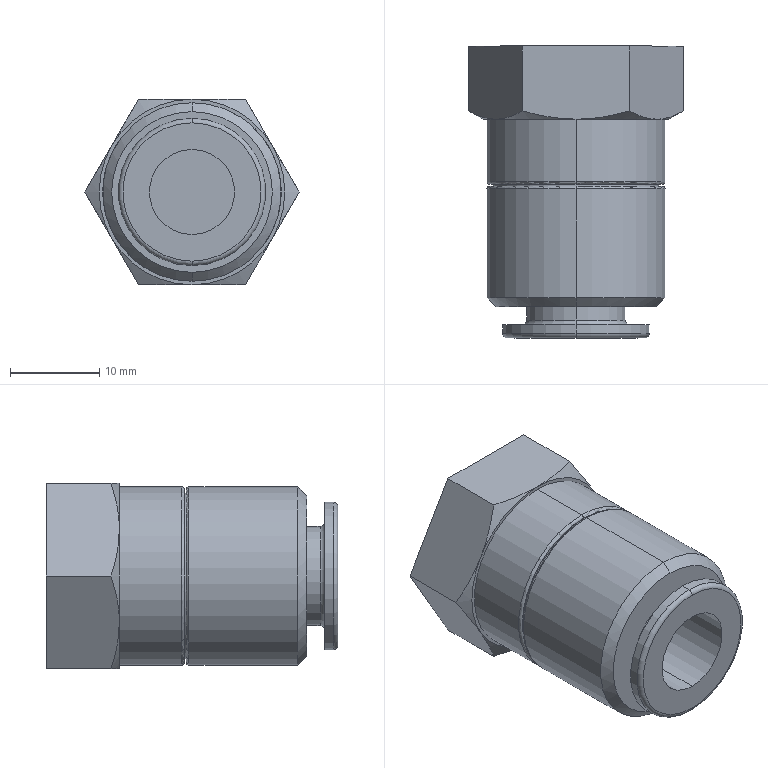Part | SolidWorks | features BaseBody 1 | 1 solid | 42 faces | box 23.995 x 32.7 x 20.78 mm | volume 9079 mm3 | plane 14 | cylinder 12 | torus 8 | cone 8 | commonest cylinder face diameters 20 x4 9.525 x2 11.1 x2 16.5 x2 18.56 x2
STEP:
#1=CARTESIAN_POINT('',(0.,-18.,4.763));
#2=VERTEX_POINT('',#1);
#3=CARTESIAN_POINT('',(0.,-18.,-4.763));
#4=VERTEX_POINT('',#3);
#5=CARTESIAN_POINT('',(0.,-18.,0.));
#6=DIRECTION('',(0.,-1.,0.));
#7=DIRECTION('',(0.,0.,-1.));
#8=AXIS2_PLACEMENT_3D('',#5,#6,#7);
#9=CIRCLE('',#8,4.763);
#10=EDGE_CURVE('',#2,#4,#9,.T.);
#11=ORIENTED_EDGE('',*,*,#10,.F.);
#12=CARTESIAN_POINT('',(0.,-32.7,4.763));
#13=VERTEX_POINT('',#12);
#14=CARTESIAN_POINT('',(0.,-32.7,4.763));
#15=DIRECTION('',(0.,-1.,0.));
#16=VECTOR('',#15,1000.);
#17=LINE('',#14,#16);
#18=EDGE_CURVE('',#2,#13,#17,.T.);
#19=ORIENTED_EDGE('',*,*,#18,.T.);
#20=CARTESIAN_POINT('',(0.,-32.7,-4.763));
#21=VERTEX_POINT('',#20);
#22=CARTESIAN_POINT('',(0.,-32.7,0.));
#23=DIRECTION('',(0.,-1.,0.));
#24=DIRECTION('',(0.,0.,-1.));
#25=AXIS2_PLACEMENT_3D('',#22,#23,#24);
#26=CIRCLE('',#25,4.763);
#27=EDGE_CURVE('',#13,#21,#26,.T.);
#28=ORIENTED_EDGE('',*,*,#27,.T.);
#29=CARTESIAN_POINT('',(0.,-32.7,-4.763));
#30=DIRECTION('',(0.,-1.,0.));
#31=VECTOR('',#30,1000.);
#32=LINE('',#29,#31);
#33=EDGE_CURVE('',#4,#21,#32,.T.);
#34=ORIENTED_EDGE('',*,*,#33,.F.);
#35=EDGE_LOOP('',(#11,#19,#28,#34));
#36=FACE_OUTER_BOUND('',#35,.T.);
#37=CARTESIAN_POINT('',(0.,-32.7,0.));
#38=DIRECTION('',(0.,-1.,0.));
#39=DIRECTION('',(0.,0.,-1.));
#40=AXIS2_PLACEMENT_3D('',#37,#38,#39);
#41=CYLINDRICAL_SURFACE('',#40,4.763);
#42=ADVANCED_FACE('',(#36),#41,.F.);
#43=CARTESIAN_POINT('',(0.,-32.2,-8.25));
#44=VERTEX_POINT('',#43);
#45=CARTESIAN_POINT('',(0.,-32.2,8.25));
#46=VERTEX_POINT('',#45);
#47=CARTESIAN_POINT('',(0.,-32.2,0.));
#48=DIRECTION('',(0.,-1.,0.));
#49=DIRECTION('',(0.,0.,-1.));
#50=AXIS2_PLACEMENT_3D('',#47,#48,#49);
#51=CIRCLE('',#50,8.25);
#52=EDGE_CURVE('',#44,#46,#51,.T.);
#53=ORIENTED_EDGE('',*,*,#52,.T.);
#54=CARTESIAN_POINT('',(0.,-32.7,7.75));
#55=VERTEX_POINT('',#54);
#56=CARTESIAN_POINT('',(0.,-32.2,7.75));
#57=DIRECTION('',(1.,0.,0.));
#58=DIRECTION('',(0.,0.,-1.));
#59=AXIS2_PLACEMENT_3D('',#56,#57,#58);
#60=CIRCLE('',#59,0.5);
#61=EDGE_CURVE('',#46,#55,#60,.T.);
#62=ORIENTED_EDGE('',*,*,#61,.T.);
#63=CARTESIAN_POINT('',(0.,-32.7,-7.75));
#64=VERTEX_POINT('',#63);
#65=CARTESIAN_POINT('',(0.,-32.7,0.));
#66=DIRECTION('',(0.,-1.,0.));
#67=DIRECTION('',(0.,0.,-1.));
#68=AXIS2_PLACEMENT_3D('',#65,#66,#67);
#69=CIRCLE('',#68,7.75);
#70=EDGE_CURVE('',#64,#55,#69,.T.);
#71=ORIENTED_EDGE('',*,*,#70,.F.);
#72=CARTESIAN_POINT('',(0.,-32.2,-7.75));
#73=DIRECTION('',(-1.,0.,0.));
#74=DIRECTION('',(0.,0.,1.));
#75=AXIS2_PLACEMENT_3D('',#72,#73,#74);
#76=CIRCLE('',#75,0.5);
#77=EDGE_CURVE('',#44,#64,#76,.T.);
#78=ORIENTED_EDGE('',*,*,#77,.F.);
#79=EDGE_LOOP('',(#53,#62,#71,#78));
#80=FACE_OUTER_BOUND('',#79,.T.);
#81=CARTESIAN_POINT('',(0.,-32.2,0.));
#82=DIRECTION('',(0.,-1.,0.));
#83=DIRECTION('',(0.,0.,-1.));
#84=AXIS2_PLACEMENT_3D('',#81,#82,#83);
#85=TOROIDAL_SURFACE('',#84,7.75,0.5);
#86=ADVANCED_FACE('',(#80),#85,.T.);
#87=CARTESIAN_POINT('',(0.,-31.2,-8.25));
#88=VERTEX_POINT('',#87);
#89=CARTESIAN_POINT('',(0.,-31.2,8.25));
#90=VERTEX_POINT('',#89);
#91=CARTESIAN_POINT('',(0.,-31.2,0.));
#92=DIRECTION('',(0.,-1.,0.));
#93=DIRECTION('',(0.,0.,-1.));
#94=AXIS2_PLACEMENT_3D('',#91,#92,#93);
#95=CIRCLE('',#94,8.25);
#96=EDGE_CURVE('',#88,#90,#95,.T.);
#97=ORIENTED_EDGE('',*,*,#96,.T.);
#98=CARTESIAN_POINT('',(0.,-32.7,8.25));
#99=DIRECTION('',(0.,-1.,0.));
#100=VECTOR('',#99,1000.);
#101=LINE('',#98,#100);
#102=EDGE_CURVE('',#90,#46,#101,.T.);
#103=ORIENTED_EDGE('',*,*,#102,.T.);
#104=ORIENTED_EDGE('',*,*,#52,.F.);
#105=CARTESIAN_POINT('',(0.,-32.7,-8.25));
#106=DIRECTION('',(0.,-1.,0.));
#107=VECTOR('',#106,1000.);
#108=LINE('',#105,#107);
#109=EDGE_CURVE('',#88,#44,#108,.T.);
#110=ORIENTED_EDGE('',*,*,#109,.F.);
#111=EDGE_LOOP('',(#97,#103,#104,#110));
#112=FACE_OUTER_BOUND('',#111,.T.);
#113=CARTESIAN_POINT('',(0.,-32.7,0.));
#114=DIRECTION('',(0.,-1.,0.));
#115=DIRECTION('',(0.,0.,-1.));
#116=AXIS2_PLACEMENT_3D('',#113,#114,#115);
#117=CYLINDRICAL_SURFACE('',#116,8.25);
#118=ADVANCED_FACE('',(#112),#117,.T.);
#119=CARTESIAN_POINT('',(0.,-31.2,6.05));
#120=VERTEX_POINT('',#119);
#121=CARTESIAN_POINT('',(0.,-31.2,-6.05));
#122=VERTEX_POINT('',#121);
#123=CARTESIAN_POINT('',(0.,-31.2,0.));
#124=DIRECTION('',(0.,-1.,0.));
#125=DIRECTION('',(0.,0.,-1.));
#126=AXIS2_PLACEMENT_3D('',#123,#124,#125);
#127=CIRCLE('',#126,6.05);
#128=EDGE_CURVE('',#120,#122,#127,.T.);
#129=ORIENTED_EDGE('',*,*,#128,.F.);
#130=CARTESIAN_POINT('',(0.,-30.7,5.55));
#131=VERTEX_POINT('',#130);
#132=CARTESIAN_POINT('',(0.,-30.7,6.05));
#133=DIRECTION('',(1.,0.,0.));
#134=DIRECTION('',(0.,0.,-1.));
#135=AXIS2_PLACEMENT_3D('',#132,#133,#134);
#136=CIRCLE('',#135,0.5);
#137=EDGE_CURVE('',#120,#131,#136,.T.);
#138=ORIENTED_EDGE('',*,*,#137,.T.);
#139=CARTESIAN_POINT('',(0.,-30.7,-5.55));
#140=VERTEX_POINT('',#139);
#141=CARTESIAN_POINT('',(0.,-30.7,0.));
#142=DIRECTION('',(0.,-1.,0.));
#143=DIRECTION('',(0.,0.,-1.));
#144=AXIS2_PLACEMENT_3D('',#141,#142,#143);
#145=CIRCLE('',#144,5.55);
#146=EDGE_CURVE('',#131,#140,#145,.T.);
#147=ORIENTED_EDGE('',*,*,#146,.T.);
#148=CARTESIAN_POINT('',(0.,-30.7,-6.05));
#149=DIRECTION('',(-1.,0.,0.));
#150=DIRECTION('',(0.,0.,1.));
#151=AXIS2_PLACEMENT_3D('',#148,#149,#150);
#152=CIRCLE('',#151,0.5);
#153=EDGE_CURVE('',#122,#140,#152,.T.);
#154=ORIENTED_EDGE('',*,*,#153,.F.);
#155=EDGE_LOOP('',(#129,#138,#147,#154));
#156=FACE_OUTER_BOUND('',#155,.T.);
#157=CARTESIAN_POINT('',(0.,-30.7,0.));
#158=DIRECTION('',(0.,-1.,0.));
#159=DIRECTION('',(0.,0.,-1.));
#160=AXIS2_PLACEMENT_3D('',#157,#158,#159);
#161=TOROIDAL_SURFACE('',#160,6.05,0.5);
#162=ADVANCED_FACE('',(#156),#161,.F.);
#163=CARTESIAN_POINT('',(0.,-29.2,-5.55));
#164=VERTEX_POINT('',#163);
#165=CARTESIAN_POINT('',(0.,-29.2,5.55));
#166=VERTEX_POINT('',#165);
#167=CARTESIAN_POINT('',(0.,-29.2,0.));
#168=DIRECTION('',(0.,-1.,0.));
#169=DIRECTION('',(0.,0.,-1.));
#170=AXIS2_PLACEMENT_3D('',#167,#168,#169);
#171=CIRCLE('',#170,5.55);
#172=EDGE_CURVE('',#164,#166,#171,.T.);
#173=ORIENTED_EDGE('',*,*,#172,.T.);
#174=CARTESIAN_POINT('',(0.,-32.7,5.55));
#175=DIRECTION('',(0.,-1.,0.));
#176=VECTOR('',#175,1000.);
#177=LINE('',#174,#176);
#178=EDGE_CURVE('',#166,#131,#177,.T.);
#179=ORIENTED_EDGE('',*,*,#178,.T.);
#180=CARTESIAN_POINT('',(0.,-30.7,0.));
#181=DIRECTION('',(0.,-1.,0.));
#182=DIRECTION('',(0.,0.,-1.));
#183=AXIS2_PLACEMENT_3D('',#180,#181,#182);
#184=CIRCLE('',#183,5.55);
#185=EDGE_CURVE('',#140,#131,#184,.T.);
#186=ORIENTED_EDGE('',*,*,#185,.F.);
#187=CARTESIAN_POINT('',(0.,-32.7,-5.55));
#188=DIRECTION('',(0.,-1.,0.));
#189=VECTOR('',#188,1000.);
#190=LINE('',#187,#189);
#191=EDGE_CURVE('',#164,#140,#190,.T.);
#192=ORIENTED_EDGE('',*,*,#191,.F.);
#193=EDGE_LOOP('',(#173,#179,#186,#192));
#194=FACE_OUTER_BOUND('',#193,.T.);
#195=CARTESIAN_POINT('',(0.,-32.7,0.));
#196=DIRECTION('',(0.,-1.,0.));
#197=DIRECTION('',(0.,0.,-1.));
#198=AXIS2_PLACEMENT_3D('',#195,#196,#197);
#199=CYLINDRICAL_SURFACE('',#198,5.55);
#200=ADVANCED_FACE('',(#194),#199,.T.);
#201=CARTESIAN_POINT('',(0.,-29.2,-9.));
#202=VERTEX_POINT('',#201);
#203=CARTESIAN_POINT('',(0.,-29.2,9.));
#204=VERTEX_POINT('',#203);
#205=CARTESIAN_POINT('',(0.,-29.2,0.));
#206=DIRECTION('',(0.,-1.,0.));
#207=DIRECTION('',(0.,0.,-1.));
#208=AXIS2_PLACEMENT_3D('',#205,#206,#207);
#209=CIRCLE('',#208,9.);
#210=EDGE_CURVE('',#202,#204,#209,.T.);
#211=ORIENTED_EDGE('',*,*,#210,.F.);
#212=CARTESIAN_POINT('',(0.,-28.2,-10.));
#213=VERTEX_POINT('',#212);
#214=CARTESIAN_POINT('',(0.,-28.2,-10.));
#215=DIRECTION('',(0.,0.7071,-0.7071));
#216=VECTOR('',#215,1000.);
#217=LINE('',#214,#216);
#218=EDGE_CURVE('',#202,#213,#217,.T.);
#219=ORIENTED_EDGE('',*,*,#218,.T.);
#220=CARTESIAN_POINT('',(0.,-28.2,10.));
#221=VERTEX_POINT('',#220);
#222=CARTESIAN_POINT('',(0.,-28.2,0.));
#223=DIRECTION('',(0.,-1.,0.));
#224=DIRECTION('',(0.,0.,-1.));
#225=AXIS2_PLACEMENT_3D('',#222,#223,#224);
#226=CIRCLE('',#225,10.);
#227=EDGE_CURVE('',#213,#221,#226,.T.);
#228=ORIENTED_EDGE('',*,*,#227,.T.);
#229=CARTESIAN_POINT('',(0.,-28.2,10.));
#230=DIRECTION('',(0.,0.7071,0.7071));
#231=VECTOR('',#230,1000.);
#232=LINE('',#229,#231);
#233=EDGE_CURVE('',#204,#221,#232,.T.);
#234=ORIENTED_EDGE('',*,*,#233,.F.);
#235=EDGE_LOOP('',(#211,#219,#228,#234));
#236=FACE_OUTER_BOUND('',#235,.T.);
#237=CARTESIAN_POINT('',(0.,-28.2,0.));
#238=DIRECTION('',(0.,1.,0.));
#239=DIRECTION('',(0.,0.,1.));
#240=AXIS2_PLACEMENT_3D('',#237,#238,#239);
#241=CONICAL_SURFACE('',#240,10.,0.7854);
#242=ADVANCED_FACE('',(#236),#241,.T.);
#243=CARTESIAN_POINT('',(0.,-16.,-10.));
#244=VERTEX_POINT('',#243);
#245=CARTESIAN_POINT('',(0.,-16.,10.));
#246=VERTEX_POINT('',#245);
#247=CARTESIAN_POINT('',(0.,-16.,0.));
#248=DIRECTION('',(0.,-1.,0.));
#249=DIRECTION('',(0.,0.,-1.));
#250=AXIS2_PLACEMENT_3D('',#247,#248,#249);
#251=CIRCLE('',#250,10.);
#252=EDGE_CURVE('',#244,#246,#251,.T.);
#253=ORIENTED_EDGE('',*,*,#252,.T.);
#254=CARTESIAN_POINT('',(0.,-32.7,10.));
#255=DIRECTION('',(0.,-1.,0.));
#256=VECTOR('',#255,1000.);
#257=LINE('',#254,#256);
#258=EDGE_CURVE('',#246,#221,#257,.T.);
#259=ORIENTED_EDGE('',*,*,#258,.T.);
#260=ORIENTED_EDGE('',*,*,#227,.F.);
#261=CARTESIAN_POINT('',(0.,-32.7,-10.));
#262=DIRECTION('',(0.,-1.,0.));
#263=VECTOR('',#262,1000.);
#264=LINE('',#261,#263);
#265=EDGE_CURVE('',#244,#213,#264,.T.);
#266=ORIENTED_EDGE('',*,*,#265,.F.);
#267=EDGE_LOOP('',(#253,#259,#260,#266));
#268=FACE_OUTER_BOUND('',#267,.T.);
#269=CARTESIAN_POINT('',(0.,-32.7,0.));
#270=DIRECTION('',(0.,-1.,0.));
#271=DIRECTION('',(0.,0.,-1.));
#272=AXIS2_PLACEMENT_3D('',#269,#270,#271);
#273=CYLINDRICAL_SURFACE('',#272,10.);
#274=ADVANCED_FACE('',(#268),#273,.T.);
#275=CARTESIAN_POINT('',(0.,-15.7,-9.7));
#276=VERTEX_POINT('',#275);
#277=CARTESIAN_POINT('',(0.,-15.7,9.7));
#278=VERTEX_POINT('',#277);
#279=CARTESIAN_POINT('',(0.,-15.7,0.));
#280=DIRECTION('',(0.,-1.,0.));
#281=DIRECTION('',(0.,0.,-1.));
#282=AXIS2_PLACEMENT_3D('',#279,#280,#281);
#283=CIRCLE('',#282,9.7);
#284=EDGE_CURVE('',#276,#278,#283,.T.);
#285=ORIENTED_EDGE('',*,*,#284,.T.);
#286=CARTESIAN_POINT('',(0.,-16.,9.7));
#287=DIRECTION('',(1.,0.,0.));
#288=DIRECTION('',(0.,0.,-1.));
#289=AXIS2_PLACEMENT_3D('',#286,#287,#288);
#290=CIRCLE('',#289,0.3);
#291=EDGE_CURVE('',#278,#246,#290,.T.);
#292=ORIENTED_EDGE('',*,*,#291,.T.);
#293=ORIENTED_EDGE('',*,*,#252,.F.);
#294=CARTESIAN_POINT('',(0.,-16.,-9.7));
#295=DIRECTION('',(-1.,0.,0.));
#296=DIRECTION('',(0.,0.,1.));
#297=AXIS2_PLACEMENT_3D('',#294,#295,#296);
#298=CIRCLE('',#297,0.3);
#299=EDGE_CURVE('',#276,#244,#298,.T.);
#300=ORIENTED_EDGE('',*,*,#299,.F.);
#301=EDGE_LOOP('',(#285,#292,#293,#300));
#302=FACE_OUTER_BOUND('',#301,.T.);
#303=CARTESIAN_POINT('',(0.,-16.,0.));
#304=DIRECTION('',(0.,-1.,0.));
#305=DIRECTION('',(0.,0.,-1.));
#306=AXIS2_PLACEMENT_3D('',#303,#304,#305);
#307=TOROIDAL_SURFACE('',#306,9.7,0.3);
#308=ADVANCED_FACE('',(#302),#307,.T.);
#309=CARTESIAN_POINT('',(0.,-15.5,-9.28));
#310=VERTEX_POINT('',#309);
#311=CARTESIAN_POINT('',(0.,-15.5,9.28));
#312=VERTEX_POINT('',#311);
#313=CARTESIAN_POINT('',(0.,-15.5,0.));
#314=DIRECTION('',(0.,-1.,0.));
#315=DIRECTION('',(0.,0.,-1.));
#316=AXIS2_PLACEMENT_3D('',#313,#314,#315);
#317=CIRCLE('',#316,9.28);
#318=EDGE_CURVE('',#310,#312,#317,.T.);
#319=ORIENTED_EDGE('',*,*,#318,.T.);
#320=CARTESIAN_POINT('',(0.,-15.7,9.28));
#321=VERTEX_POINT('',#320);
#322=CARTESIAN_POINT('',(0.,-32.7,9.28));
#323=DIRECTION('',(0.,-1.,0.));
#324=VECTOR('',#323,1000.);
#325=LINE('',#322,#324);
#326=EDGE_CURVE('',#312,#321,#325,.T.);
#327=ORIENTED_EDGE('',*,*,#326,.T.);
#328=CARTESIAN_POINT('',(0.,-15.7,-9.28));
#329=VERTEX_POINT('',#328);
#330=CARTESIAN_POINT('',(0.,-15.7,0.));
#331=DIRECTION('',(0.,-1.,0.));
#332=DIRECTION('',(0.,0.,-1.));
#333=AXIS2_PLACEMENT_3D('',#330,#331,#332);
#334=CIRCLE('',#333,9.28);
#335=EDGE_CURVE('',#329,#321,#334,.T.);
#336=ORIENTED_EDGE('',*,*,#335,.F.);
#337=CARTESIAN_POINT('',(0.,-32.7,-9.28));
#338=DIRECTION('',(0.,-1.,0.));
#339=VECTOR('',#338,1000.);
#340=LINE('',#337,#339);
#341=EDGE_CURVE('',#310,#329,#340,.T.);
#342=ORIENTED_EDGE('',*,*,#341,.F.);
#343=EDGE_LOOP('',(#319,#327,#336,#342));
#344=FACE_OUTER_BOUND('',#343,.T.);
#345=CARTESIAN_POINT('',(0.,-32.7,0.));
#346=DIRECTION('',(0.,-1.,0.));
#347=DIRECTION('',(0.,0.,-1.));
#348=AXIS2_PLACEMENT_3D('',#345,#346,#347);
#349=CYLINDRICAL_SURFACE('',#348,9.28);
#350=ADVANCED_FACE('',(#344),#349,.T.);
#351=CARTESIAN_POINT('',(0.,-15.2,-10.));
#352=VERTEX_POINT('',#351);
#353=CARTESIAN_POINT('',(0.,-15.2,10.));
#354=VERTEX_POINT('',#353);
#355=CARTESIAN_POINT('',(0.,-15.2,0.));
#356=DIRECTION('',(0.,-1.,0.));
#357=DIRECTION('',(0.,0.,-1.));
#358=AXIS2_PLACEMENT_3D('',#355,#356,#357);
#359=CIRCLE('',#358,10.);
#360=EDGE_CURVE('',#352,#354,#359,.T.);
#361=ORIENTED_EDGE('',*,*,#360,.T.);
#362=CARTESIAN_POINT('',(0.,-15.5,9.7));
#363=VERTEX_POINT('',#362);
#364=CARTESIAN_POINT('',(0.,-15.2,9.7));
#365=DIRECTION('',(1.,0.,0.));
#366=DIRECTION('',(0.,0.,-1.));
#367=AXIS2_PLACEMENT_3D('',#364,#365,#366);
#368=CIRCLE('',#367,0.3);
#369=EDGE_CURVE('',#354,#363,#368,.T.);
#370=ORIENTED_EDGE('',*,*,#369,.T.);
#371=CARTESIAN_POINT('',(0.,-15.5,-9.7));
#372=VERTEX_POINT('',#371);
#373=CARTESIAN_POINT('',(0.,-15.5,0.));
#374=DIRECTION('',(0.,-1.,0.));
#375=DIRECTION('',(0.,0.,-1.));
#376=AXIS2_PLACEMENT_3D('',#373,#374,#375);
#377=CIRCLE('',#376,9.7);
#378=EDGE_CURVE('',#372,#363,#377,.T.);
#379=ORIENTED_EDGE('',*,*,#378,.F.);
#380=CARTESIAN_POINT('',(0.,-15.2,-9.7));
#381=DIRECTION('',(-1.,0.,0.));
#382=DIRECTION('',(0.,0.,1.));
#383=AXIS2_PLACEMENT_3D('',#380,#381,#382);
#384=CIRCLE('',#383,0.3);
#385=EDGE_CURVE('',#352,#372,#384,.T.);
#386=ORIENTED_EDGE('',*,*,#385,.F.);
#387=EDGE_LOOP('',(#361,#370,#379,#386));
#388=FACE_OUTER_BOUND('',#387,.T.);
#389=CARTESIAN_POINT('',(0.,-15.2,0.));
#390=DIRECTION('',(0.,-1.,0.));
#391=DIRECTION('',(0.,0.,-1.));
#392=AXIS2_PLACEMENT_3D('',#389,#390,#391);
#393=TOROIDAL_SURFACE('',#392,9.7,0.3);
#394=ADVANCED_FACE('',(#388),#393,.T.);
#395=CARTESIAN_POINT('',(0.,-8.2,-10.));
#396=VERTEX_POINT('',#395);
#397=CARTESIAN_POINT('',(0.,-8.2,10.));
#398=VERTEX_POINT('',#397);
#399=CARTESIAN_POINT('',(0.,-8.2,0.));
#400=DIRECTION('',(0.,-1.,0.));
#401=DIRECTION('',(0.,0.,-1.));
#402=AXIS2_PLACEMENT_3D('',#399,#400,#401);
#403=CIRCLE('',#402,10.);
#404=EDGE_CURVE('',#396,#398,#403,.T.);
#405=ORIENTED_EDGE('',*,*,#404,.T.);
#406=CARTESIAN_POINT('',(0.,-32.7,10.));
#407=DIRECTION('',(0.,-1.,0.));
#408=VECTOR('',#407,1000.);
#409=LINE('',#406,#408);
#410=EDGE_CURVE('',#398,#354,#409,.T.);
#411=ORIENTED_EDGE('',*,*,#410,.T.);
#412=ORIENTED_EDGE('',*,*,#360,.F.);
#413=CARTESIAN_POINT('',(0.,-32.7,-10.));
#414=DIRECTION('',(0.,-1.,0.));
#415=VECTOR('',#414,1000.);
#416=LINE('',#413,#415);
#417=EDGE_CURVE('',#396,#352,#416,.T.);
#418=ORIENTED_EDGE('',*,*,#417,.F.);
#419=EDGE_LOOP('',(#405,#411,#412,#418));
#420=FACE_OUTER_BOUND('',#419,.T.);
#421=CARTESIAN_POINT('',(0.,-32.7,0.));
#422=DIRECTION('',(0.,-1.,0.));
#423=DIRECTION('',(0.,0.,-1.));
#424=AXIS2_PLACEMENT_3D('',#421,#422,#423);
#425=CYLINDRICAL_SURFACE('',#424,10.);
#426=ADVANCED_FACE('',(#420),#425,.T.);
#427=CARTESIAN_POINT('',(8.998,-8.2,-5.195));
#428=VERTEX_POINT('',#427);
#429=CARTESIAN_POINT('',(5.999,-7.272,-10.39));
#430=VERTEX_POINT('',#429);
#431=CARTESIAN_POINT('',(8.998,-8.2,-5.195));
#432=CARTESIAN_POINT('',(8.488,-8.2,-6.078));
#433=CARTESIAN_POINT('',(7.983,-8.112,-6.954));
#434=CARTESIAN_POINT('',(6.98,-7.788,-8.69));
#435=CARTESIAN_POINT('',(6.486,-7.554,-9.545));
#436=CARTESIAN_POINT('',(5.999,-7.272,-10.39));
#437=B_SPLINE_CURVE_WITH_KNOTS('',3,(#431,#432,#433,#434,#435,#436),.UNSPECIFIED.,.F.,.F.,(4,2,4),(6.07,9.093,12.117),.UNSPECIFIED.);
#438=EDGE_CURVE('',#428,#430,#437,.T.);
#439=ORIENTED_EDGE('',*,*,#438,.F.);
#440=CARTESIAN_POINT('',(0.,-8.2,-10.39));
#441=VERTEX_POINT('',#440);
#442=CARTESIAN_POINT('',(0.,-8.2,0.));
#443=DIRECTION('',(0.,-1.,0.));
#444=DIRECTION('',(0.,0.,-1.));
#445=AXIS2_PLACEMENT_3D('',#442,#443,#444);
#446=CIRCLE('',#445,10.39);
#447=EDGE_CURVE('',#441,#428,#446,.T.);
#448=ORIENTED_EDGE('',*,*,#447,.F.);
#449=CARTESIAN_POINT('',(5.999,-7.272,-10.39));
#450=CARTESIAN_POINT('',(5.023,-7.554,-10.39));
#451=CARTESIAN_POINT('',(4.039,-7.787,-10.39));
#452=CARTESIAN_POINT('',(2.539,-8.03,-10.39));
#453=CARTESIAN_POINT('',(2.038,-8.093,-10.39));
#454=CARTESIAN_POINT('',(1.024,-8.178,-10.39));
#455=CARTESIAN_POINT('',(0.5136,-8.2,-10.39));
#456=CARTESIAN_POINT('',(0.,-8.2,-10.39));
#457=B_SPLINE_CURVE_WITH_KNOTS('',3,(#449,#450,#451,#452,#453,#454,#455,#456),.UNSPECIFIED.,.F.,.F.,(4,2,2,4),(13.621,16.671,18.196,19.721),.UNSPECIFIED.);
#458=EDGE_CURVE('',#430,#441,#457,.T.);
#459=ORIENTED_EDGE('',*,*,#458,.F.);
#460=EDGE_LOOP('',(#439,#448,#459));
#461=FACE_OUTER_BOUND('',#460,.T.);
#462=CARTESIAN_POINT('',(0.,-4.601,0.));
#463=DIRECTION('',(0.,1.,0.));
#464=DIRECTION('',(0.,0.,1.));
#465=AXIS2_PLACEMENT_3D('',#462,#463,#464);
#466=CONICAL_SURFACE('',#465,16.624,1.047);
#467=ADVANCED_FACE('',(#461),#466,.T.);
#468=CARTESIAN_POINT('',(11.997,-7.272,0.));
#469=VERTEX_POINT('',#468);
#470=CARTESIAN_POINT('',(11.997,-7.272,0.));
#471=CARTESIAN_POINT('',(11.509,-7.554,-0.8459));
#472=CARTESIAN_POINT('',(11.014,-7.788,-1.703));
#473=CARTESIAN_POINT('',(10.263,-8.031,-3.005));
#474=CARTESIAN_POINT('',(10.013,-8.093,-3.437));
#475=CARTESIAN_POINT('',(9.507,-8.178,-4.313));
#476=CARTESIAN_POINT('',(9.252,-8.2,-4.754));
#477=CARTESIAN_POINT('',(8.998,-8.2,-5.195));
#478=B_SPLINE_CURVE_WITH_KNOTS('',3,(#470,#471,#472,#473,#474,#475,#476,#477),.UNSPECIFIED.,.F.,.F.,(4,2,2,4),(0.0002381,3.035,4.552,6.07),.UNSPECIFIED.);
#479=EDGE_CURVE('',#469,#428,#478,.T.);
#480=ORIENTED_EDGE('',*,*,#479,.T.);
#481=ORIENTED_EDGE('',*,*,#438,.T.);
#482=CARTESIAN_POINT('',(5.999,0.,-10.39));
#483=VERTEX_POINT('',#482);
#484=CARTESIAN_POINT('',(5.999,-7.272,-10.39));
#485=DIRECTION('',(0.,1.,0.));
#486=VECTOR('',#485,1000.);
#487=LINE('',#484,#486);
#488=EDGE_CURVE('',#430,#483,#487,.T.);
#489=ORIENTED_EDGE('',*,*,#488,.T.);
#490=CARTESIAN_POINT('',(11.997,0.,0.));
#491=VERTEX_POINT('',#490);
#492=CARTESIAN_POINT('',(11.997,0.,0.));
#493=DIRECTION('',(-0.5,0.,-0.866));
#494=VECTOR('',#493,1000.);
#495=LINE('',#492,#494);
#496=EDGE_CURVE('',#491,#483,#495,.T.);
#497=ORIENTED_EDGE('',*,*,#496,.F.);
#498=CARTESIAN_POINT('',(11.997,-7.272,0.));
#499=DIRECTION('',(0.,1.,0.));
#500=VECTOR('',#499,1000.);
#501=LINE('',#498,#500);
#502=EDGE_CURVE('',#469,#491,#501,.T.);
#503=ORIENTED_EDGE('',*,*,#502,.F.);
#504=EDGE_LOOP('',(#480,#481,#489,#497,#503));
#505=FACE_OUTER_BOUND('',#504,.T.);
#506=CARTESIAN_POINT('',(11.997,-9.,0.));
#507=DIRECTION('',(0.866,0.,-0.5));
#508=DIRECTION('',(-0.5,0.,-0.866));
#509=AXIS2_PLACEMENT_3D('',#506,#507,#508);
#510=PLANE('',#509);
#511=ADVANCED_FACE('',(#505),#510,.T.);
#512=ORIENTED_EDGE('',*,*,#404,.F.);
#513=CARTESIAN_POINT('',(0.,-8.2,0.));
#514=DIRECTION('',(0.,-1.,0.));
#515=DIRECTION('',(0.,0.,-1.));
#516=AXIS2_PLACEMENT_3D('',#513,#514,#515);
#517=CIRCLE('',#516,10.);
#518=EDGE_CURVE('',#398,#396,#517,.T.);
#519=ORIENTED_EDGE('',*,*,#518,.F.);
#520=EDGE_LOOP('',(#512,#519));
#521=FACE_BOUND('',#520,.T.);
#522=ORIENTED_EDGE('',*,*,#447,.T.);
#523=CARTESIAN_POINT('',(8.998,-8.2,5.195));
#524=VERTEX_POINT('',#523);
#525=CARTESIAN_POINT('',(0.,-8.2,0.));
#526=DIRECTION('',(0.,-1.,0.));
#527=DIRECTION('',(0.866,0.,-0.5));
#528=AXIS2_PLACEMENT_3D('',#525,#526,#527);
#529=CIRCLE('',#528,10.39);
#530=EDGE_CURVE('',#428,#524,#529,.T.);
#531=ORIENTED_EDGE('',*,*,#530,.T.);
#532=CARTESIAN_POINT('',(0.,-8.2,10.39));
#533=VERTEX_POINT('',#532);
#534=CARTESIAN_POINT('',(0.,-8.2,0.));
#535=DIRECTION('',(0.,-1.,0.));
#536=DIRECTION('',(0.866,0.,0.5));
#537=AXIS2_PLACEMENT_3D('',#534,#535,#536);
#538=CIRCLE('',#537,10.39);
#539=EDGE_CURVE('',#524,#533,#538,.T.);
#540=ORIENTED_EDGE('',*,*,#539,.T.);
#541=CARTESIAN_POINT('',(-8.998,-8.2,5.195));
#542=VERTEX_POINT('',#541);
#543=CARTESIAN_POINT('',(0.,-8.2,0.));
#544=DIRECTION('',(0.,-1.,0.));
#545=DIRECTION('',(0.,0.,1.));
#546=AXIS2_PLACEMENT_3D('',#543,#544,#545);
#547=CIRCLE('',#546,10.39);
#548=EDGE_CURVE('',#533,#542,#547,.T.);
#549=ORIENTED_EDGE('',*,*,#548,.T.);
#550=CARTESIAN_POINT('',(-8.998,-8.2,-5.195));
#551=VERTEX_POINT('',#550);
#552=CARTESIAN_POINT('',(0.,-8.2,0.));
#553=DIRECTION('',(0.,-1.,0.));
#554=DIRECTION('',(-0.866,0.,0.5));
#555=AXIS2_PLACEMENT_3D('',#552,#553,#554);
#556=CIRCLE('',#555,10.39);
#557=EDGE_CURVE('',#542,#551,#556,.T.);
#558=ORIENTED_EDGE('',*,*,#557,.T.);
#559=CARTESIAN_POINT('',(0.,-8.2,0.));
#560=DIRECTION('',(0.,-1.,0.));
#561=DIRECTION('',(-0.866,0.,-0.5));
#562=AXIS2_PLACEMENT_3D('',#559,#560,#561);
#563=CIRCLE('',#562,10.39);
#564=EDGE_CURVE('',#551,#441,#563,.T.);
#565=ORIENTED_EDGE('',*,*,#564,.T.);
#566=EDGE_LOOP('',(#522,#531,#540,#549,#558,#565));
#567=FACE_OUTER_BOUND('',#566,.T.);
#568=CARTESIAN_POINT('',(10.39,-8.2,0.));
#569=DIRECTION('',(0.,1.,0.));
#570=DIRECTION('',(0.,0.,1.));
#571=AXIS2_PLACEMENT_3D('',#568,#569,#570);
#572=PLANE('',#571);
#573=ADVANCED_FACE('',(#521,#567),#572,.F.);
#574=ORIENTED_EDGE('',*,*,#458,.T.);
#575=CARTESIAN_POINT('',(-5.999,-7.272,-10.39));
#576=VERTEX_POINT('',#575);
#577=CARTESIAN_POINT('',(0.,-8.2,-10.39));
#578=CARTESIAN_POINT('',(-0.5108,-8.2,-10.39));
#579=CARTESIAN_POINT('',(-1.023,-8.178,-10.39));
#580=CARTESIAN_POINT('',(-2.037,-8.093,-10.39));
#581=CARTESIAN_POINT('',(-2.537,-8.03,-10.39));
#582=CARTESIAN_POINT('',(-4.039,-7.787,-10.39));
#583=CARTESIAN_POINT('',(-5.024,-7.553,-10.39));
#584=CARTESIAN_POINT('',(-5.999,-7.272,-10.39));
#585=B_SPLINE_CURVE_WITH_KNOTS('',3,(#577,#578,#579,#580,#581,#582,#583,#584),.UNSPECIFIED.,.F.,.F.,(4,2,2,4),(19.721,21.248,22.774,25.827),.UNSPECIFIED.);
#586=EDGE_CURVE('',#441,#576,#585,.T.);
#587=ORIENTED_EDGE('',*,*,#586,.T.);
#588=CARTESIAN_POINT('',(-5.999,0.,-10.39));
#589=VERTEX_POINT('',#588);
#590=CARTESIAN_POINT('',(-5.999,-7.272,-10.39));
#591=DIRECTION('',(0.,1.,0.));
#592=VECTOR('',#591,1000.);
#593=LINE('',#590,#592);
#594=EDGE_CURVE('',#576,#589,#593,.T.);
#595=ORIENTED_EDGE('',*,*,#594,.T.);
#596=CARTESIAN_POINT('',(5.999,0.,-10.39));
#597=DIRECTION('',(-1.,0.,0.));
#598=VECTOR('',#597,1000.);
#599=LINE('',#596,#598);
#600=EDGE_CURVE('',#483,#589,#599,.T.);
#601=ORIENTED_EDGE('',*,*,#600,.F.);
#602=ORIENTED_EDGE('',*,*,#488,.F.);
#603=EDGE_LOOP('',(#574,#587,#595,#601,#602));
#604=FACE_OUTER_BOUND('',#603,.T.);
#605=CARTESIAN_POINT('',(5.999,-9.,-10.39));
#606=DIRECTION('',(0.,0.,-1.));
#607=DIRECTION('',(-1.,0.,0.));
#608=AXIS2_PLACEMENT_3D('',#605,#606,#607);
#609=PLANE('',#608);
#610=ADVANCED_FACE('',(#604),#609,.T.);
#611=CARTESIAN_POINT('',(8.998,-8.2,5.195));
#612=CARTESIAN_POINT('',(9.508,-8.2,4.312));
#613=CARTESIAN_POINT('',(10.013,-8.112,3.436));
#614=CARTESIAN_POINT('',(11.016,-7.788,1.7));
#615=CARTESIAN_POINT('',(11.51,-7.554,0.8448));
#616=CARTESIAN_POINT('',(11.997,-7.272,0.));
#617=B_SPLINE_CURVE_WITH_KNOTS('',3,(#611,#612,#613,#614,#615,#616),.UNSPECIFIED.,.F.,.F.,(4,2,4),(6.07,9.093,12.117),.UNSPECIFIED.);
#618=EDGE_CURVE('',#524,#469,#617,.T.);
#619=ORIENTED_EDGE('',*,*,#618,.F.);
#620=ORIENTED_EDGE('',*,*,#530,.F.);
#621=ORIENTED_EDGE('',*,*,#479,.F.);
#622=EDGE_LOOP('',(#619,#620,#621));
#623=FACE_OUTER_BOUND('',#622,.T.);
#624=CARTESIAN_POINT('',(0.,-4.601,0.));
#625=DIRECTION('',(0.,1.,0.));
#626=DIRECTION('',(0.,0.,1.));
#627=AXIS2_PLACEMENT_3D('',#624,#625,#626);
#628=CONICAL_SURFACE('',#627,16.624,1.047);
#629=ADVANCED_FACE('',(#623),#628,.T.);
#630=CARTESIAN_POINT('',(5.999,0.,10.39));
#631=VERTEX_POINT('',#630);
#632=CARTESIAN_POINT('',(5.999,0.,10.39));
#633=DIRECTION('',(0.5,0.,-0.866));
#634=VECTOR('',#633,1000.);
#635=LINE('',#632,#634);
#636=EDGE_CURVE('',#631,#491,#635,.T.);
#637=ORIENTED_EDGE('',*,*,#636,.T.);
#638=ORIENTED_EDGE('',*,*,#496,.T.);
#639=ORIENTED_EDGE('',*,*,#600,.T.);
#640=CARTESIAN_POINT('',(-11.997,0.,0.));
#641=VERTEX_POINT('',#640);
#642=CARTESIAN_POINT('',(-5.999,0.,-10.39));
#643=DIRECTION('',(-0.5,0.,0.866));
#644=VECTOR('',#643,1000.);
#645=LINE('',#642,#644);
#646=EDGE_CURVE('',#589,#641,#645,.T.);
#647=ORIENTED_EDGE('',*,*,#646,.T.);
#648=CARTESIAN_POINT('',(-5.999,0.,10.39));
#649=VERTEX_POINT('',#648);
#650=CARTESIAN_POINT('',(-11.997,0.,0.));
#651=DIRECTION('',(0.5,0.,0.866));
#652=VECTOR('',#651,1000.);
#653=LINE('',#650,#652);
#654=EDGE_CURVE('',#641,#649,#653,.T.);
#655=ORIENTED_EDGE('',*,*,#654,.T.);
#656=CARTESIAN_POINT('',(-5.999,0.,10.39));
#657=DIRECTION('',(1.,0.,0.));
#658=VECTOR('',#657,1000.);
#659=LINE('',#656,#658);
#660=EDGE_CURVE('',#649,#631,#659,.T.);
#661=ORIENTED_EDGE('',*,*,#660,.T.);
#662=EDGE_LOOP('',(#637,#638,#639,#647,#655,#661));
#663=FACE_OUTER_BOUND('',#662,.T.);
#664=CARTESIAN_POINT('',(0.,0.,0.));
#665=DIRECTION('',(0.,-1.,0.));
#666=DIRECTION('',(0.,0.,-1.));
#667=AXIS2_PLACEMENT_3D('',#664,#665,#666);
#668=PLANE('',#667);
#669=ADVANCED_FACE('',(#663),#668,.F.);
#670=CARTESIAN_POINT('',(5.999,-7.272,10.39));
#671=VERTEX_POINT('',#670);
#672=CARTESIAN_POINT('',(5.999,-7.272,10.39));
#673=CARTESIAN_POINT('',(6.487,-7.554,9.544));
#674=CARTESIAN_POINT('',(6.982,-7.788,8.687));
#675=CARTESIAN_POINT('',(7.733,-8.031,7.385));
#676=CARTESIAN_POINT('',(7.983,-8.093,6.953));
#677=CARTESIAN_POINT('',(8.489,-8.178,6.077));
#678=CARTESIAN_POINT('',(8.744,-8.2,5.636));
#679=CARTESIAN_POINT('',(8.998,-8.2,5.195));
#680=B_SPLINE_CURVE_WITH_KNOTS('',3,(#672,#673,#674,#675,#676,#677,#678,#679),.UNSPECIFIED.,.F.,.F.,(4,2,2,4),(0.0002381,3.035,4.552,6.07),.UNSPECIFIED.);
#681=EDGE_CURVE('',#671,#524,#680,.T.);
#682=ORIENTED_EDGE('',*,*,#681,.T.);
#683=ORIENTED_EDGE('',*,*,#618,.T.);
#684=ORIENTED_EDGE('',*,*,#502,.T.);
#685=ORIENTED_EDGE('',*,*,#636,.F.);
#686=CARTESIAN_POINT('',(5.999,-7.272,10.39));
#687=DIRECTION('',(0.,1.,0.));
#688=VECTOR('',#687,1000.);
#689=LINE('',#686,#688);
#690=EDGE_CURVE('',#671,#631,#689,.T.);
#691=ORIENTED_EDGE('',*,*,#690,.F.);
#692=EDGE_LOOP('',(#682,#683,#684,#685,#691));
#693=FACE_OUTER_BOUND('',#692,.T.);
#694=CARTESIAN_POINT('',(5.999,-9.,10.39));
#695=DIRECTION('',(0.866,0.,0.5));
#696=DIRECTION('',(0.5,0.,-0.866));
#697=AXIS2_PLACEMENT_3D('',#694,#695,#696);
#698=PLANE('',#697);
#699=ADVANCED_FACE('',(#693),#698,.T.);
#700=ORIENTED_EDGE('',*,*,#410,.F.);
#701=ORIENTED_EDGE('',*,*,#518,.T.);
#702=ORIENTED_EDGE('',*,*,#417,.T.);
#703=CARTESIAN_POINT('',(0.,-15.2,0.));
#704=DIRECTION('',(0.,-1.,0.));
#705=DIRECTION('',(0.,0.,-1.));
#706=AXIS2_PLACEMENT_3D('',#703,#704,#705);
#707=CIRCLE('',#706,10.);
#708=EDGE_CURVE('',#354,#352,#707,.T.);
#709=ORIENTED_EDGE('',*,*,#708,.F.);
#710=EDGE_LOOP('',(#700,#701,#702,#709));
#711=FACE_OUTER_BOUND('',#710,.T.);
#712=CARTESIAN_POINT('',(0.,-32.7,0.));
#713=DIRECTION('',(0.,-1.,0.));
#714=DIRECTION('',(0.,0.,-1.));
#715=AXIS2_PLACEMENT_3D('',#712,#713,#714);
#716=CYLINDRICAL_SURFACE('',#715,10.);
#717=ADVANCED_FACE('',(#711),#716,.T.);
#718=ORIENTED_EDGE('',*,*,#681,.F.);
#719=CARTESIAN_POINT('',(0.,-8.2,10.39));
#720=CARTESIAN_POINT('',(0.5108,-8.2,10.39));
#721=CARTESIAN_POINT('',(1.023,-8.178,10.39));
#722=CARTESIAN_POINT('',(2.037,-8.093,10.39));
#723=CARTESIAN_POINT('',(2.537,-8.03,10.39));
#724=CARTESIAN_POINT('',(4.039,-7.787,10.39));
#725=CARTESIAN_POINT('',(5.024,-7.553,10.39));
#726=CARTESIAN_POINT('',(5.999,-7.272,10.39));
#727=B_SPLINE_CURVE_WITH_KNOTS('',3,(#719,#720,#721,#722,#723,#724,#725,#726),.UNSPECIFIED.,.F.,.F.,(4,2,2,4),(19.721,21.248,22.774,25.827),.UNSPECIFIED.);
#728=EDGE_CURVE('',#533,#671,#727,.T.);
#729=ORIENTED_EDGE('',*,*,#728,.F.);
#730=ORIENTED_EDGE('',*,*,#539,.F.);
#731=EDGE_LOOP('',(#718,#729,#730));
#732=FACE_OUTER_BOUND('',#731,.T.);
#733=CARTESIAN_POINT('',(0.,-4.601,0.));
#734=DIRECTION('',(0.,1.,0.));
#735=DIRECTION('',(0.,0.,1.));
#736=AXIS2_PLACEMENT_3D('',#733,#734,#735);
#737=CONICAL_SURFACE('',#736,16.624,1.047);
#738=ADVANCED_FACE('',(#732),#737,.T.);
#739=CARTESIAN_POINT('',(-5.999,-7.272,10.39));
#740=VERTEX_POINT('',#739);
#741=CARTESIAN_POINT('',(-5.999,-7.272,10.39));
#742=CARTESIAN_POINT('',(-5.023,-7.554,10.39));
#743=CARTESIAN_POINT('',(-4.039,-7.787,10.39));
#744=CARTESIAN_POINT('',(-2.539,-8.03,10.39));
#745=CARTESIAN_POINT('',(-2.038,-8.093,10.39));
#746=CARTESIAN_POINT('',(-1.024,-8.178,10.39));
#747=CARTESIAN_POINT('',(-0.5136,-8.2,10.39));
#748=CARTESIAN_POINT('',(0.,-8.2,10.39));
#749=B_SPLINE_CURVE_WITH_KNOTS('',3,(#741,#742,#743,#744,#745,#746,#747,#748),.UNSPECIFIED.,.F.,.F.,(4,2,2,4),(13.621,16.671,18.196,19.721),.UNSPECIFIED.);
#750=EDGE_CURVE('',#740,#533,#749,.T.);
#751=ORIENTED_EDGE('',*,*,#750,.F.);
#752=CARTESIAN_POINT('',(-8.998,-8.2,5.195));
#753=CARTESIAN_POINT('',(-8.488,-8.2,6.078));
#754=CARTESIAN_POINT('',(-7.983,-8.112,6.954));
#755=CARTESIAN_POINT('',(-6.98,-7.788,8.69));
#756=CARTESIAN_POINT('',(-6.486,-7.554,9.545));
#757=CARTESIAN_POINT('',(-5.999,-7.272,10.39));
#758=B_SPLINE_CURVE_WITH_KNOTS('',3,(#752,#753,#754,#755,#756,#757),.UNSPECIFIED.,.F.,.F.,(4,2,4),(6.07,9.093,12.117),.UNSPECIFIED.);
#759=EDGE_CURVE('',#542,#740,#758,.T.);
#760=ORIENTED_EDGE('',*,*,#759,.F.);
#761=ORIENTED_EDGE('',*,*,#548,.F.);
#762=EDGE_LOOP('',(#751,#760,#761));
#763=FACE_OUTER_BOUND('',#762,.T.);
#764=CARTESIAN_POINT('',(0.,-4.601,0.));
#765=DIRECTION('',(0.,1.,0.));
#766=DIRECTION('',(0.,0.,1.));
#767=AXIS2_PLACEMENT_3D('',#764,#765,#766);
#768=CONICAL_SURFACE('',#767,16.624,1.047);
#769=ADVANCED_FACE('',(#763),#768,.T.);
#770=CARTESIAN_POINT('',(-11.997,-7.272,0.));
#771=VERTEX_POINT('',#770);
#772=CARTESIAN_POINT('',(-8.998,-8.2,-5.195));
#773=CARTESIAN_POINT('',(-9.508,-8.2,-4.312));
#774=CARTESIAN_POINT('',(-10.013,-8.112,-3.436));
#775=CARTESIAN_POINT('',(-11.016,-7.788,-1.7));
#776=CARTESIAN_POINT('',(-11.51,-7.554,-0.8448));
#777=CARTESIAN_POINT('',(-11.997,-7.272,0.));
#778=B_SPLINE_CURVE_WITH_KNOTS('',3,(#772,#773,#774,#775,#776,#777),.UNSPECIFIED.,.F.,.F.,(4,2,4),(6.07,9.093,12.117),.UNSPECIFIED.);
#779=EDGE_CURVE('',#551,#771,#778,.T.);
#780=ORIENTED_EDGE('',*,*,#779,.F.);
#781=ORIENTED_EDGE('',*,*,#557,.F.);
#782=CARTESIAN_POINT('',(-11.997,-7.272,0.));
#783=CARTESIAN_POINT('',(-11.509,-7.554,0.8459));
#784=CARTESIAN_POINT('',(-11.014,-7.788,1.703));
#785=CARTESIAN_POINT('',(-10.263,-8.031,3.005));
#786=CARTESIAN_POINT('',(-10.013,-8.093,3.437));
#787=CARTESIAN_POINT('',(-9.507,-8.178,4.313));
#788=CARTESIAN_POINT('',(-9.252,-8.2,4.754));
#789=CARTESIAN_POINT('',(-8.998,-8.2,5.195));
#790=B_SPLINE_CURVE_WITH_KNOTS('',3,(#782,#783,#784,#785,#786,#787,#788,#789),.UNSPECIFIED.,.F.,.F.,(4,2,2,4),(0.0002381,3.035,4.552,6.07),.UNSPECIFIED.);
#791=EDGE_CURVE('',#771,#542,#790,.T.);
#792=ORIENTED_EDGE('',*,*,#791,.F.);
#793=EDGE_LOOP('',(#780,#781,#792));
#794=FACE_OUTER_BOUND('',#793,.T.);
#795=CARTESIAN_POINT('',(0.,-4.601,0.));
#796=DIRECTION('',(0.,1.,0.));
#797=DIRECTION('',(0.,0.,1.));
#798=AXIS2_PLACEMENT_3D('',#795,#796,#797);
#799=CONICAL_SURFACE('',#798,16.624,1.047);
#800=ADVANCED_FACE('',(#794),#799,.T.);
#801=ORIENTED_EDGE('',*,*,#586,.F.);
#802=ORIENTED_EDGE('',*,*,#564,.F.);
#803=CARTESIAN_POINT('',(-5.999,-7.272,-10.39));
#804=CARTESIAN_POINT('',(-6.487,-7.554,-9.544));
#805=CARTESIAN_POINT('',(-6.982,-7.788,-8.687));
#806=CARTESIAN_POINT('',(-7.733,-8.031,-7.385));
#807=CARTESIAN_POINT('',(-7.983,-8.093,-6.953));
#808=CARTESIAN_POINT('',(-8.489,-8.178,-6.077));
#809=CARTESIAN_POINT('',(-8.744,-8.2,-5.636));
#810=CARTESIAN_POINT('',(-8.998,-8.2,-5.195));
#811=B_SPLINE_CURVE_WITH_KNOTS('',3,(#803,#804,#805,#806,#807,#808,#809,#810),.UNSPECIFIED.,.F.,.F.,(4,2,2,4),(0.0002381,3.035,4.552,6.07),.UNSPECIFIED.);
#812=EDGE_CURVE('',#576,#551,#811,.T.);
#813=ORIENTED_EDGE('',*,*,#812,.F.);
#814=EDGE_LOOP('',(#801,#802,#813));
#815=FACE_OUTER_BOUND('',#814,.T.);
#816=CARTESIAN_POINT('',(0.,-4.601,0.));
#817=DIRECTION('',(0.,1.,0.));
#818=DIRECTION('',(0.,0.,1.));
#819=AXIS2_PLACEMENT_3D('',#816,#817,#818);
#820=CONICAL_SURFACE('',#819,16.624,1.047);
#821=ADVANCED_FACE('',(#815),#820,.T.);
#822=ORIENTED_EDGE('',*,*,#812,.T.);
#823=ORIENTED_EDGE('',*,*,#779,.T.);
#824=CARTESIAN_POINT('',(-11.997,-7.272,0.));
#825=DIRECTION('',(0.,1.,0.));
#826=VECTOR('',#825,1000.);
#827=LINE('',#824,#826);
#828=EDGE_CURVE('',#771,#641,#827,.T.);
#829=ORIENTED_EDGE('',*,*,#828,.T.);
#830=ORIENTED_EDGE('',*,*,#646,.F.);
#831=ORIENTED_EDGE('',*,*,#594,.F.);
#832=EDGE_LOOP('',(#822,#823,#829,#830,#831));
#833=FACE_OUTER_BOUND('',#832,.T.);
#834=CARTESIAN_POINT('',(-5.999,-9.,-10.39));
#835=DIRECTION('',(-0.866,0.,-0.5));
#836=DIRECTION('',(-0.5,0.,0.866));
#837=AXIS2_PLACEMENT_3D('',#834,#835,#836);
#838=PLANE('',#837);
#839=ADVANCED_FACE('',(#833),#838,.T.);
#840=ORIENTED_EDGE('',*,*,#791,.T.);
#841=ORIENTED_EDGE('',*,*,#759,.T.);
#842=CARTESIAN_POINT('',(-5.999,-7.272,10.39));
#843=DIRECTION('',(0.,1.,0.));
#844=VECTOR('',#843,1000.);
#845=LINE('',#842,#844);
#846=EDGE_CURVE('',#740,#649,#845,.T.);
#847=ORIENTED_EDGE('',*,*,#846,.T.);
#848=ORIENTED_EDGE('',*,*,#654,.F.);
#849=ORIENTED_EDGE('',*,*,#828,.F.);
#850=EDGE_LOOP('',(#840,#841,#847,#848,#849));
#851=FACE_OUTER_BOUND('',#850,.T.);
#852=CARTESIAN_POINT('',(-11.997,-9.,0.));
#853=DIRECTION('',(-0.866,0.,0.5));
#854=DIRECTION('',(0.5,0.,0.866));
#855=AXIS2_PLACEMENT_3D('',#852,#853,#854);
#856=PLANE('',#855);
#857=ADVANCED_FACE('',(#851),#856,.T.);
#858=ORIENTED_EDGE('',*,*,#750,.T.);
#859=ORIENTED_EDGE('',*,*,#728,.T.);
#860=ORIENTED_EDGE('',*,*,#690,.T.);
#861=ORIENTED_EDGE('',*,*,#660,.F.);
#862=ORIENTED_EDGE('',*,*,#846,.F.);
#863=EDGE_LOOP('',(#858,#859,#860,#861,#862));
#864=FACE_OUTER_BOUND('',#863,.T.);
#865=CARTESIAN_POINT('',(-5.999,-9.,10.39));
#866=DIRECTION('',(0.,0.,1.));
#867=DIRECTION('',(1.,0.,0.));
#868=AXIS2_PLACEMENT_3D('',#865,#866,#867);
#869=PLANE('',#868);
#870=ADVANCED_FACE('',(#864),#869,.T.);
#871=ORIENTED_EDGE('',*,*,#369,.F.);
#872=ORIENTED_EDGE('',*,*,#708,.T.);
#873=ORIENTED_EDGE('',*,*,#385,.T.);
#874=CARTESIAN_POINT('',(0.,-15.5,0.));
#875=DIRECTION('',(0.,-1.,0.));
#876=DIRECTION('',(0.,0.,-1.));
#877=AXIS2_PLACEMENT_3D('',#874,#875,#876);
#878=CIRCLE('',#877,9.7);
#879=EDGE_CURVE('',#363,#372,#878,.T.);
#880=ORIENTED_EDGE('',*,*,#879,.F.);
#881=EDGE_LOOP('',(#871,#872,#873,#880));
#882=FACE_OUTER_BOUND('',#881,.T.);
#883=CARTESIAN_POINT('',(0.,-15.2,0.));
#884=DIRECTION('',(0.,-1.,0.));
#885=DIRECTION('',(0.,0.,-1.));
#886=AXIS2_PLACEMENT_3D('',#883,#884,#885);
#887=TOROIDAL_SURFACE('',#886,9.7,0.3);
#888=ADVANCED_FACE('',(#882),#887,.T.);
#889=ORIENTED_EDGE('',*,*,#318,.F.);
#890=CARTESIAN_POINT('',(0.,-15.5,0.));
#891=DIRECTION('',(0.,-1.,0.));
#892=DIRECTION('',(0.,0.,-1.));
#893=AXIS2_PLACEMENT_3D('',#890,#891,#892);
#894=CIRCLE('',#893,9.28);
#895=EDGE_CURVE('',#312,#310,#894,.T.);
#896=ORIENTED_EDGE('',*,*,#895,.F.);
#897=EDGE_LOOP('',(#889,#896));
#898=FACE_BOUND('',#897,.T.);
#899=ORIENTED_EDGE('',*,*,#378,.T.);
#900=ORIENTED_EDGE('',*,*,#879,.T.);
#901=EDGE_LOOP('',(#899,#900));
#902=FACE_OUTER_BOUND('',#901,.T.);
#903=CARTESIAN_POINT('',(9.7,-15.5,0.));
#904=DIRECTION('',(0.,1.,0.));
#905=DIRECTION('',(0.,0.,1.));
#906=AXIS2_PLACEMENT_3D('',#903,#904,#905);
#907=PLANE('',#906);
#908=ADVANCED_FACE('',(#898,#902),#907,.F.);
#909=ORIENTED_EDGE('',*,*,#326,.F.);
#910=ORIENTED_EDGE('',*,*,#895,.T.);
#911=ORIENTED_EDGE('',*,*,#341,.T.);
#912=CARTESIAN_POINT('',(0.,-15.7,0.));
#913=DIRECTION('',(0.,-1.,0.));
#914=DIRECTION('',(0.,0.,-1.));
#915=AXIS2_PLACEMENT_3D('',#912,#913,#914);
#916=CIRCLE('',#915,9.28);
#917=EDGE_CURVE('',#321,#329,#916,.T.);
#918=ORIENTED_EDGE('',*,*,#917,.F.);
#919=EDGE_LOOP('',(#909,#910,#911,#918));
#920=FACE_OUTER_BOUND('',#919,.T.);
#921=CARTESIAN_POINT('',(0.,-32.7,0.));
#922=DIRECTION('',(0.,-1.,0.));
#923=DIRECTION('',(0.,0.,-1.));
#924=AXIS2_PLACEMENT_3D('',#921,#922,#923);
#925=CYLINDRICAL_SURFACE('',#924,9.28);
#926=ADVANCED_FACE('',(#920),#925,.T.);
#927=ORIENTED_EDGE('',*,*,#284,.F.);
#928=CARTESIAN_POINT('',(0.,-15.7,0.));
#929=DIRECTION('',(0.,-1.,0.));
#930=DIRECTION('',(0.,0.,-1.));
#931=AXIS2_PLACEMENT_3D('',#928,#929,#930);
#932=CIRCLE('',#931,9.7);
#933=EDGE_CURVE('',#278,#276,#932,.T.);
#934=ORIENTED_EDGE('',*,*,#933,.F.);
#935=EDGE_LOOP('',(#927,#934));
#936=FACE_OUTER_BOUND('',#935,.T.);
#937=ORIENTED_EDGE('',*,*,#335,.T.);
#938=ORIENTED_EDGE('',*,*,#917,.T.);
#939=EDGE_LOOP('',(#937,#938));
#940=FACE_BOUND('',#939,.T.);
#941=CARTESIAN_POINT('',(9.28,-15.7,0.));
#942=DIRECTION('',(0.,-1.,0.));
#943=DIRECTION('',(0.,0.,-1.));
#944=AXIS2_PLACEMENT_3D('',#941,#942,#943);
#945=PLANE('',#944);
#946=ADVANCED_FACE('',(#936,#940),#945,.F.);
#947=ORIENTED_EDGE('',*,*,#291,.F.);
#948=ORIENTED_EDGE('',*,*,#933,.T.);
#949=ORIENTED_EDGE('',*,*,#299,.T.);
#950=CARTESIAN_POINT('',(0.,-16.,0.));
#951=DIRECTION('',(0.,-1.,0.));
#952=DIRECTION('',(0.,0.,-1.));
#953=AXIS2_PLACEMENT_3D('',#950,#951,#952);
#954=CIRCLE('',#953,10.);
#955=EDGE_CURVE('',#246,#244,#954,.T.);
#956=ORIENTED_EDGE('',*,*,#955,.F.);
#957=EDGE_LOOP('',(#947,#948,#949,#956));
#958=FACE_OUTER_BOUND('',#957,.T.);
#959=CARTESIAN_POINT('',(0.,-16.,0.));
#960=DIRECTION('',(0.,-1.,0.));
#961=DIRECTION('',(0.,0.,-1.));
#962=AXIS2_PLACEMENT_3D('',#959,#960,#961);
#963=TOROIDAL_SURFACE('',#962,9.7,0.3);
#964=ADVANCED_FACE('',(#958),#963,.T.);
#965=ORIENTED_EDGE('',*,*,#258,.F.);
#966=ORIENTED_EDGE('',*,*,#955,.T.);
#967=ORIENTED_EDGE('',*,*,#265,.T.);
#968=CARTESIAN_POINT('',(0.,-28.2,0.));
#969=DIRECTION('',(0.,-1.,0.));
#970=DIRECTION('',(0.,0.,-1.));
#971=AXIS2_PLACEMENT_3D('',#968,#969,#970);
#972=CIRCLE('',#971,10.);
#973=EDGE_CURVE('',#221,#213,#972,.T.);
#974=ORIENTED_EDGE('',*,*,#973,.F.);
#975=EDGE_LOOP('',(#965,#966,#967,#974));
#976=FACE_OUTER_BOUND('',#975,.T.);
#977=CARTESIAN_POINT('',(0.,-32.7,0.));
#978=DIRECTION('',(0.,-1.,0.));
#979=DIRECTION('',(0.,0.,-1.));
#980=AXIS2_PLACEMENT_3D('',#977,#978,#979);
#981=CYLINDRICAL_SURFACE('',#980,10.);
#982=ADVANCED_FACE('',(#976),#981,.T.);
#983=ORIENTED_EDGE('',*,*,#218,.F.);
#984=CARTESIAN_POINT('',(0.,-29.2,0.));
#985=DIRECTION('',(0.,-1.,0.));
#986=DIRECTION('',(0.,0.,-1.));
#987=AXIS2_PLACEMENT_3D('',#984,#985,#986);
#988=CIRCLE('',#987,9.);
#989=EDGE_CURVE('',#204,#202,#988,.T.);
#990=ORIENTED_EDGE('',*,*,#989,.F.);
#991=ORIENTED_EDGE('',*,*,#233,.T.);
#992=ORIENTED_EDGE('',*,*,#973,.T.);
#993=EDGE_LOOP('',(#983,#990,#991,#992));
#994=FACE_OUTER_BOUND('',#993,.T.);
#995=CARTESIAN_POINT('',(0.,-28.2,0.));
#996=DIRECTION('',(0.,1.,0.));
#997=DIRECTION('',(0.,0.,1.));
#998=AXIS2_PLACEMENT_3D('',#995,#996,#997);
#999=CONICAL_SURFACE('',#998,10.,0.7854);
#1000=ADVANCED_FACE('',(#994),#999,.T.);
#1001=ORIENTED_EDGE('',*,*,#172,.F.);
#1002=CARTESIAN_POINT('',(0.,-29.2,0.));
#1003=DIRECTION('',(0.,-1.,0.));
#1004=DIRECTION('',(0.,0.,-1.));
#1005=AXIS2_PLACEMENT_3D('',#1002,#1003,#1004);
#1006=CIRCLE('',#1005,5.55);
#1007=EDGE_CURVE('',#166,#164,#1006,.T.);
#1008=ORIENTED_EDGE('',*,*,#1007,.F.);
#1009=EDGE_LOOP('',(#1001,#1008));
#1010=FACE_BOUND('',#1009,.T.);
#1011=ORIENTED_EDGE('',*,*,#989,.T.);
#1012=ORIENTED_EDGE('',*,*,#210,.T.);
#1013=EDGE_LOOP('',(#1011,#1012));
#1014=FACE_OUTER_BOUND('',#1013,.T.);
#1015=CARTESIAN_POINT('',(9.,-29.2,0.));
#1016=DIRECTION('',(0.,1.,0.));
#1017=DIRECTION('',(0.,0.,1.));
#1018=AXIS2_PLACEMENT_3D('',#1015,#1016,#1017);
#1019=PLANE('',#1018);
#1020=ADVANCED_FACE('',(#1010,#1014),#1019,.F.);
#1021=ORIENTED_EDGE('',*,*,#178,.F.);
#1022=ORIENTED_EDGE('',*,*,#1007,.T.);
#1023=ORIENTED_EDGE('',*,*,#191,.T.);
#1024=ORIENTED_EDGE('',*,*,#146,.F.);
#1025=EDGE_LOOP('',(#1021,#1022,#1023,#1024));
#1026=FACE_OUTER_BOUND('',#1025,.T.);
#1027=CARTESIAN_POINT('',(0.,-32.7,0.));
#1028=DIRECTION('',(0.,-1.,0.));
#1029=DIRECTION('',(0.,0.,-1.));
#1030=AXIS2_PLACEMENT_3D('',#1027,#1028,#1029);
#1031=CYLINDRICAL_SURFACE('',#1030,5.55);
#1032=ADVANCED_FACE('',(#1026),#1031,.T.);
#1033=ORIENTED_EDGE('',*,*,#137,.F.);
#1034=CARTESIAN_POINT('',(0.,-31.2,0.));
#1035=DIRECTION('',(0.,-1.,0.));
#1036=DIRECTION('',(0.,0.,-1.));
#1037=AXIS2_PLACEMENT_3D('',#1034,#1035,#1036);
#1038=CIRCLE('',#1037,6.05);
#1039=EDGE_CURVE('',#122,#120,#1038,.T.);
#1040=ORIENTED_EDGE('',*,*,#1039,.F.);
#1041=ORIENTED_EDGE('',*,*,#153,.T.);
#1042=ORIENTED_EDGE('',*,*,#185,.T.);
#1043=EDGE_LOOP('',(#1033,#1040,#1041,#1042));
#1044=FACE_OUTER_BOUND('',#1043,.T.);
#1045=CARTESIAN_POINT('',(0.,-30.7,0.));
#1046=DIRECTION('',(0.,-1.,0.));
#1047=DIRECTION('',(0.,0.,-1.));
#1048=AXIS2_PLACEMENT_3D('',#1045,#1046,#1047);
#1049=TOROIDAL_SURFACE('',#1048,6.05,0.5);
#1050=ADVANCED_FACE('',(#1044),#1049,.F.);
#1051=ORIENTED_EDGE('',*,*,#96,.F.);
#1052=CARTESIAN_POINT('',(0.,-31.2,0.));
#1053=DIRECTION('',(0.,-1.,0.));
#1054=DIRECTION('',(0.,0.,-1.));
#1055=AXIS2_PLACEMENT_3D('',#1052,#1053,#1054);
#1056=CIRCLE('',#1055,8.25);
#1057=EDGE_CURVE('',#90,#88,#1056,.T.);
#1058=ORIENTED_EDGE('',*,*,#1057,.F.);
#1059=EDGE_LOOP('',(#1051,#1058));
#1060=FACE_OUTER_BOUND('',#1059,.T.);
#1061=ORIENTED_EDGE('',*,*,#1039,.T.);
#1062=ORIENTED_EDGE('',*,*,#128,.T.);
#1063=EDGE_LOOP('',(#1061,#1062));
#1064=FACE_BOUND('',#1063,.T.);
#1065=CARTESIAN_POINT('',(6.05,-31.2,0.));
#1066=DIRECTION('',(0.,-1.,0.));
#1067=DIRECTION('',(0.,0.,-1.));
#1068=AXIS2_PLACEMENT_3D('',#1065,#1066,#1067);
#1069=PLANE('',#1068);
#1070=ADVANCED_FACE('',(#1060,#1064),#1069,.F.);
#1071=ORIENTED_EDGE('',*,*,#102,.F.);
#1072=ORIENTED_EDGE('',*,*,#1057,.T.);
#1073=ORIENTED_EDGE('',*,*,#109,.T.);
#1074=CARTESIAN_POINT('',(0.,-32.2,0.));
#1075=DIRECTION('',(0.,-1.,0.));
#1076=DIRECTION('',(0.,0.,-1.));
#1077=AXIS2_PLACEMENT_3D('',#1074,#1075,#1076);
#1078=CIRCLE('',#1077,8.25);
#1079=EDGE_CURVE('',#46,#44,#1078,.T.);
#1080=ORIENTED_EDGE('',*,*,#1079,.F.);
#1081=EDGE_LOOP('',(#1071,#1072,#1073,#1080));
#1082=FACE_OUTER_BOUND('',#1081,.T.);
#1083=CARTESIAN_POINT('',(0.,-32.7,0.));
#1084=DIRECTION('',(0.,-1.,0.));
#1085=DIRECTION('',(0.,0.,-1.));
#1086=AXIS2_PLACEMENT_3D('',#1083,#1084,#1085);
#1087=CYLINDRICAL_SURFACE('',#1086,8.25);
#1088=ADVANCED_FACE('',(#1082),#1087,.T.);
#1089=ORIENTED_EDGE('',*,*,#61,.F.);
#1090=ORIENTED_EDGE('',*,*,#1079,.T.);
#1091=ORIENTED_EDGE('',*,*,#77,.T.);
#1092=CARTESIAN_POINT('',(0.,-32.7,0.));
#1093=DIRECTION('',(0.,-1.,0.));
#1094=DIRECTION('',(0.,0.,-1.));
#1095=AXIS2_PLACEMENT_3D('',#1092,#1093,#1094);
#1096=CIRCLE('',#1095,7.75);
#1097=EDGE_CURVE('',#55,#64,#1096,.T.);
#1098=ORIENTED_EDGE('',*,*,#1097,.F.);
#1099=EDGE_LOOP('',(#1089,#1090,#1091,#1098));
#1100=FACE_OUTER_BOUND('',#1099,.T.);
#1101=CARTESIAN_POINT('',(0.,-32.2,0.));
#1102=DIRECTION('',(0.,-1.,0.));
#1103=DIRECTION('',(0.,0.,-1.));
#1104=AXIS2_PLACEMENT_3D('',#1101,#1102,#1103);
#1105=TOROIDAL_SURFACE('',#1104,7.75,0.5);
#1106=ADVANCED_FACE('',(#1100),#1105,.T.);
#1107=CARTESIAN_POINT('',(0.,-32.7,0.));
#1108=DIRECTION('',(0.,-1.,0.));
#1109=DIRECTION('',(0.,0.,-1.));
#1110=AXIS2_PLACEMENT_3D('',#1107,#1108,#1109);
#1111=CIRCLE('',#1110,4.763);
#1112=EDGE_CURVE('',#21,#13,#1111,.T.);
#1113=ORIENTED_EDGE('',*,*,#1112,.F.);
#1114=ORIENTED_EDGE('',*,*,#27,.F.);
#1115=EDGE_LOOP('',(#1113,#1114));
#1116=FACE_BOUND('',#1115,.T.);
#1117=ORIENTED_EDGE('',*,*,#70,.T.);
#1118=ORIENTED_EDGE('',*,*,#1097,.T.);
#1119=EDGE_LOOP('',(#1117,#1118));
#1120=FACE_OUTER_BOUND('',#1119,.T.);
#1121=CARTESIAN_POINT('',(7.75,-32.7,0.));
#1122=DIRECTION('',(0.,1.,0.));
#1123=DIRECTION('',(0.,0.,1.));
#1124=AXIS2_PLACEMENT_3D('',#1121,#1122,#1123);
#1125=PLANE('',#1124);
#1126=ADVANCED_FACE('',(#1116,#1120),#1125,.F.);
#1127=ORIENTED_EDGE('',*,*,#18,.F.);
#1128=CARTESIAN_POINT('',(0.,-18.,0.));
#1129=DIRECTION('',(0.,-1.,0.));
#1130=DIRECTION('',(0.,0.,-1.));
#1131=AXIS2_PLACEMENT_3D('',#1128,#1129,#1130);
#1132=CIRCLE('',#1131,4.763);
#1133=EDGE_CURVE('',#4,#2,#1132,.T.);
#1134=ORIENTED_EDGE('',*,*,#1133,.F.);
#1135=ORIENTED_EDGE('',*,*,#33,.T.);
#1136=ORIENTED_EDGE('',*,*,#1112,.T.);
#1137=EDGE_LOOP('',(#1127,#1134,#1135,#1136));
#1138=FACE_OUTER_BOUND('',#1137,.T.);
#1139=CARTESIAN_POINT('',(0.,-32.7,0.));
#1140=DIRECTION('',(0.,-1.,0.));
#1141=DIRECTION('',(0.,0.,-1.));
#1142=AXIS2_PLACEMENT_3D('',#1139,#1140,#1141);
#1143=CYLINDRICAL_SURFACE('',#1142,4.763);
#1144=ADVANCED_FACE('',(#1138),#1143,.F.);
#1145=ORIENTED_EDGE('',*,*,#1133,.T.);
#1146=ORIENTED_EDGE('',*,*,#10,.T.);
#1147=EDGE_LOOP('',(#1145,#1146));
#1148=FACE_OUTER_BOUND('',#1147,.T.);
#1149=CARTESIAN_POINT('',(4.763,-18.,0.));
#1150=DIRECTION('',(0.,1.,0.));
#1151=DIRECTION('',(0.,0.,1.));
#1152=AXIS2_PLACEMENT_3D('',#1149,#1150,#1151);
#1153=PLANE('',#1152);
#1154=ADVANCED_FACE('',(#1148),#1153,.F.);
#1155=CLOSED_SHELL('',(#42,#86,#118,#162,#200,#242,#274,#308,#350,#394,#426,#467,#511,#573,#610,#629,#669,#699,#717,#738,#769,#800,#821,#839,#857,#870,#888,#908,#926,#946,#964,#982,#1000,#1020,#1032,#1050,#1070,#1088,#1106,#1126,#1144,#1154));
#1156=MANIFOLD_SOLID_BREP('',#1155);
#1157=CARTESIAN_POINT('',(0.,0.,0.));
#1158=DIRECTION('',(0.,0.,1.));
#1159=DIRECTION('',(1.,0.,0.));
#1160=AXIS2_PLACEMENT_3D('',#1157,#1158,#1159);
#1161=(LENGTH_UNIT()NAMED_UNIT(*)SI_UNIT(.MILLI.,.METRE.));
#1162=UNCERTAINTY_MEASURE_WITH_UNIT(LENGTH_MEASURE(0.00001),#1161,'','');
#1163=(NAMED_UNIT(*)PLANE_ANGLE_UNIT()SI_UNIT($,.RADIAN.));
#1164=(NAMED_UNIT(*)SI_UNIT($,.STERADIAN.)SOLID_ANGLE_UNIT());
#1165=(GEOMETRIC_REPRESENTATION_CONTEXT(3)GLOBAL_UNCERTAINTY_ASSIGNED_CONTEXT((#1162))GLOBAL_UNIT_ASSIGNED_CONTEXT((#1161,#1163,#1164))REPRESENTATION_CONTEXT('',''));
#1166=ADVANCED_BREP_SHAPE_REPRESENTATION('',(#1156,#1160),#1165);